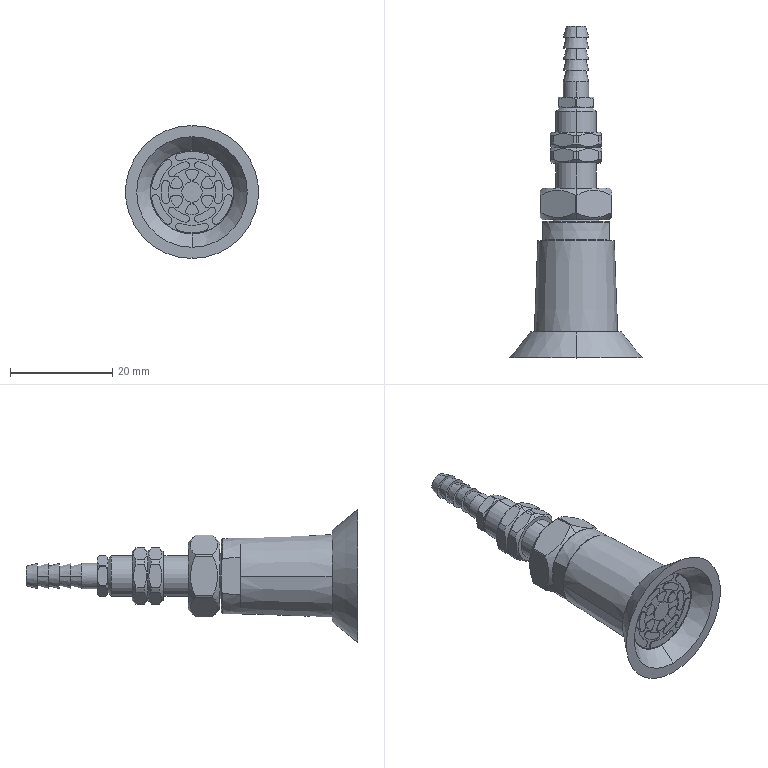Part | SolidWorks | 4 solids | 283 faces | box 26 x 64.9 x 26 mm | volume 7528 mm3 | cylinder 138 | plane 83 | cone 62 | commonest cylinder face diameters 0.888 x14 11 x14 1.421 x13 1.464 x11 1.776 x9 8 x9